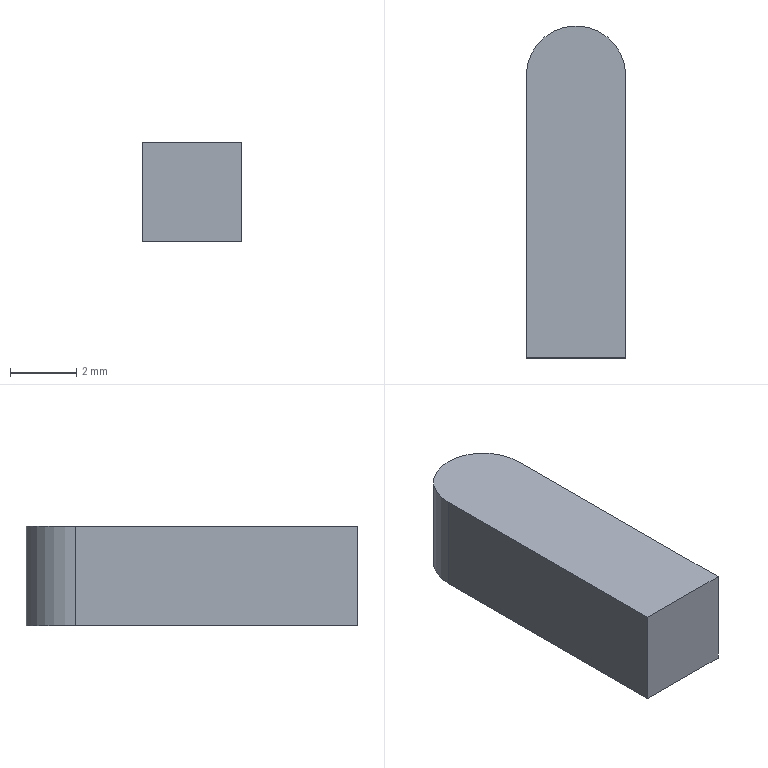Part | NX | features DATUM_CSYS 2, EXTRUDE 1, SKETCH 1 | 1 solid | 6 faces | box 3 x 10 x 3 mm | volume 87.103 mm3 | plane 5 | cylinder 1 | commonest cylinder face diameters 3 x1
STEP:
#1=CARTESIAN_POINT('',(-1.5,8.5,0.));
#2=VERTEX_POINT('',#1);
#3=CARTESIAN_POINT('',(-1.5,0.,0.));
#4=VERTEX_POINT('',#3);
#5=CARTESIAN_POINT('',(-1.5,8.5,0.));
#6=DIRECTION('',(0.,-1.,0.));
#7=VECTOR('',#6,1000.);
#8=LINE('',#5,#7);
#9=EDGE_CURVE('',#2,#4,#8,.T.);
#10=ORIENTED_EDGE('',*,*,#9,.T.);
#11=CARTESIAN_POINT('',(-1.5,0.,3.));
#12=VERTEX_POINT('',#11);
#13=CARTESIAN_POINT('',(-1.5,0.,3.));
#14=DIRECTION('',(0.,0.,-1.));
#15=VECTOR('',#14,1000.);
#16=LINE('',#13,#15);
#17=EDGE_CURVE('',#12,#4,#16,.T.);
#18=ORIENTED_EDGE('',*,*,#17,.F.);
#19=CARTESIAN_POINT('',(-1.5,8.5,3.));
#20=VERTEX_POINT('',#19);
#21=CARTESIAN_POINT('',(-1.5,8.5,3.));
#22=DIRECTION('',(0.,-1.,0.));
#23=VECTOR('',#22,1000.);
#24=LINE('',#21,#23);
#25=EDGE_CURVE('',#20,#12,#24,.T.);
#26=ORIENTED_EDGE('',*,*,#25,.F.);
#27=CARTESIAN_POINT('',(-1.5,8.5,3.));
#28=DIRECTION('',(0.,0.,-1.));
#29=VECTOR('',#28,1000.);
#30=LINE('',#27,#29);
#31=EDGE_CURVE('',#20,#2,#30,.T.);
#32=ORIENTED_EDGE('',*,*,#31,.T.);
#33=EDGE_LOOP('',(#10,#18,#26,#32));
#34=FACE_BOUND('',#33,.T.);
#35=CARTESIAN_POINT('',(-1.5,8.5,3.));
#36=DIRECTION('',(1.,0.,0.));
#37=DIRECTION('',(0.,1.,0.));
#38=AXIS2_PLACEMENT_3D('',#35,#36,#37);
#39=PLANE('',#38);
#40=ADVANCED_FACE('',(#34),#39,.F.);
#41=CARTESIAN_POINT('',(1.5,0.,0.));
#42=VERTEX_POINT('',#41);
#43=CARTESIAN_POINT('',(-1.5,0.,0.));
#44=DIRECTION('',(1.,0.,0.));
#45=VECTOR('',#44,1000.);
#46=LINE('',#43,#45);
#47=EDGE_CURVE('',#4,#42,#46,.T.);
#48=ORIENTED_EDGE('',*,*,#47,.T.);
#49=CARTESIAN_POINT('',(1.5,0.,3.));
#50=VERTEX_POINT('',#49);
#51=CARTESIAN_POINT('',(1.5,0.,3.));
#52=DIRECTION('',(0.,0.,-1.));
#53=VECTOR('',#52,1000.);
#54=LINE('',#51,#53);
#55=EDGE_CURVE('',#50,#42,#54,.T.);
#56=ORIENTED_EDGE('',*,*,#55,.F.);
#57=CARTESIAN_POINT('',(-1.5,0.,3.));
#58=DIRECTION('',(1.,0.,0.));
#59=VECTOR('',#58,1000.);
#60=LINE('',#57,#59);
#61=EDGE_CURVE('',#12,#50,#60,.T.);
#62=ORIENTED_EDGE('',*,*,#61,.F.);
#63=ORIENTED_EDGE('',*,*,#17,.T.);
#64=EDGE_LOOP('',(#48,#56,#62,#63));
#65=FACE_BOUND('',#64,.T.);
#66=CARTESIAN_POINT('',(-1.5,0.,3.));
#67=DIRECTION('',(0.,1.,0.));
#68=DIRECTION('',(0.,0.,1.));
#69=AXIS2_PLACEMENT_3D('',#66,#67,#68);
#70=PLANE('',#69);
#71=ADVANCED_FACE('',(#65),#70,.F.);
#72=CARTESIAN_POINT('',(1.5,8.5,0.));
#73=VERTEX_POINT('',#72);
#74=CARTESIAN_POINT('',(1.5,0.,0.));
#75=DIRECTION('',(0.,1.,0.));
#76=VECTOR('',#75,1000.);
#77=LINE('',#74,#76);
#78=EDGE_CURVE('',#42,#73,#77,.T.);
#79=ORIENTED_EDGE('',*,*,#78,.T.);
#80=CARTESIAN_POINT('',(1.5,8.5,3.));
#81=VERTEX_POINT('',#80);
#82=CARTESIAN_POINT('',(1.5,8.5,3.));
#83=DIRECTION('',(0.,0.,-1.));
#84=VECTOR('',#83,1000.);
#85=LINE('',#82,#84);
#86=EDGE_CURVE('',#81,#73,#85,.T.);
#87=ORIENTED_EDGE('',*,*,#86,.F.);
#88=CARTESIAN_POINT('',(1.5,0.,3.));
#89=DIRECTION('',(0.,1.,0.));
#90=VECTOR('',#89,1000.);
#91=LINE('',#88,#90);
#92=EDGE_CURVE('',#50,#81,#91,.T.);
#93=ORIENTED_EDGE('',*,*,#92,.F.);
#94=ORIENTED_EDGE('',*,*,#55,.T.);
#95=EDGE_LOOP('',(#79,#87,#93,#94));
#96=FACE_BOUND('',#95,.T.);
#97=CARTESIAN_POINT('',(1.5,0.,3.));
#98=DIRECTION('',(-1.,0.,0.));
#99=DIRECTION('',(0.,-1.,0.));
#100=AXIS2_PLACEMENT_3D('',#97,#98,#99);
#101=PLANE('',#100);
#102=ADVANCED_FACE('',(#96),#101,.F.);
#103=CARTESIAN_POINT('',(0.,8.5,0.));
#104=DIRECTION('',(0.,0.,1.));
#105=DIRECTION('',(1.,0.,0.));
#106=AXIS2_PLACEMENT_3D('',#103,#104,#105);
#107=CIRCLE('',#106,1.5);
#108=EDGE_CURVE('',#73,#2,#107,.T.);
#109=ORIENTED_EDGE('',*,*,#108,.T.);
#110=ORIENTED_EDGE('',*,*,#31,.F.);
#111=CARTESIAN_POINT('',(0.,8.5,3.));
#112=DIRECTION('',(0.,0.,1.));
#113=DIRECTION('',(1.,0.,0.));
#114=AXIS2_PLACEMENT_3D('',#111,#112,#113);
#115=CIRCLE('',#114,1.5);
#116=EDGE_CURVE('',#81,#20,#115,.T.);
#117=ORIENTED_EDGE('',*,*,#116,.F.);
#118=ORIENTED_EDGE('',*,*,#86,.T.);
#119=EDGE_LOOP('',(#109,#110,#117,#118));
#120=FACE_BOUND('',#119,.T.);
#121=CARTESIAN_POINT('',(0.,8.5,3.));
#122=DIRECTION('',(0.,0.,-1.));
#123=DIRECTION('',(-1.,0.,0.));
#124=AXIS2_PLACEMENT_3D('',#121,#122,#123);
#125=CYLINDRICAL_SURFACE('',#124,1.5);
#126=ADVANCED_FACE('',(#120),#125,.T.);
#127=ORIENTED_EDGE('',*,*,#25,.T.);
#128=ORIENTED_EDGE('',*,*,#61,.T.);
#129=ORIENTED_EDGE('',*,*,#92,.T.);
#130=ORIENTED_EDGE('',*,*,#116,.T.);
#131=EDGE_LOOP('',(#127,#128,#129,#130));
#132=FACE_BOUND('',#131,.T.);
#133=CARTESIAN_POINT('',(0.,8.5,3.));
#134=DIRECTION('',(0.,0.,1.));
#135=DIRECTION('',(1.,0.,0.));
#136=AXIS2_PLACEMENT_3D('',#133,#134,#135);
#137=PLANE('',#136);
#138=ADVANCED_FACE('',(#132),#137,.T.);
#139=ORIENTED_EDGE('',*,*,#9,.F.);
#140=ORIENTED_EDGE('',*,*,#108,.F.);
#141=ORIENTED_EDGE('',*,*,#78,.F.);
#142=ORIENTED_EDGE('',*,*,#47,.F.);
#143=EDGE_LOOP('',(#139,#140,#141,#142));
#144=FACE_BOUND('',#143,.T.);
#145=CARTESIAN_POINT('',(0.,8.5,0.));
#146=DIRECTION('',(0.,0.,1.));
#147=DIRECTION('',(1.,0.,0.));
#148=AXIS2_PLACEMENT_3D('',#145,#146,#147);
#149=PLANE('',#148);
#150=ADVANCED_FACE('',(#144),#149,.F.);
#151=CLOSED_SHELL('',(#40,#71,#102,#126,#138,#150));
#152=MANIFOLD_SOLID_BREP('',#151);
#153=(LENGTH_UNIT()NAMED_UNIT(*)SI_UNIT(.MILLI.,.METRE.));
#154=UNCERTAINTY_MEASURE_WITH_UNIT(LENGTH_MEASURE(0.00001),#153,'','');
#155=(NAMED_UNIT(*)PLANE_ANGLE_UNIT()SI_UNIT($,.RADIAN.));
#156=(NAMED_UNIT(*)SI_UNIT($,.STERADIAN.)SOLID_ANGLE_UNIT());
#157=(GEOMETRIC_REPRESENTATION_CONTEXT(3)GLOBAL_UNCERTAINTY_ASSIGNED_CONTEXT((#154))GLOBAL_UNIT_ASSIGNED_CONTEXT((#153,#155,#156))REPRESENTATION_CONTEXT('',''));
#158=ADVANCED_BREP_SHAPE_REPRESENTATION('',(#152),#157);